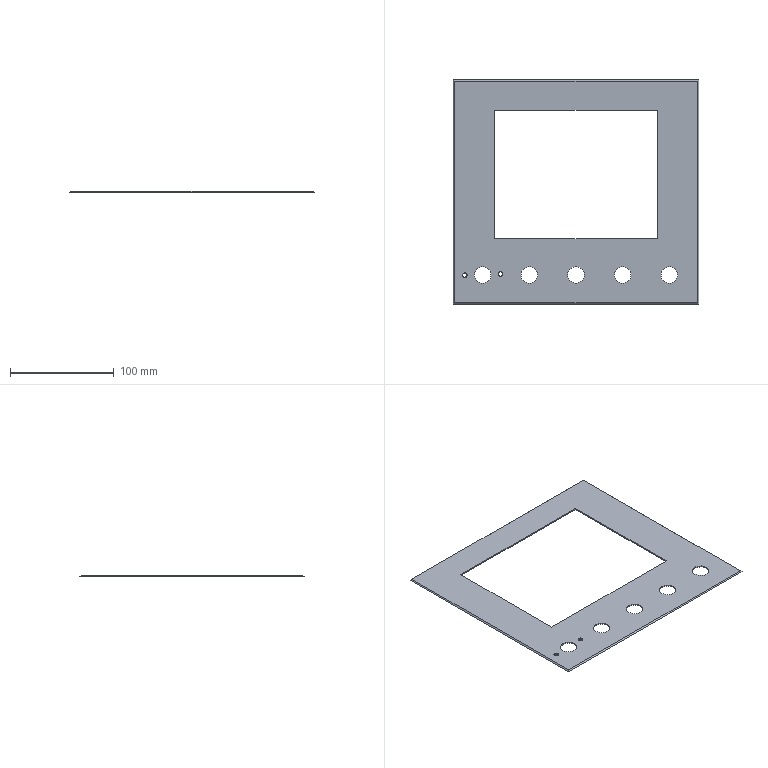Part | NX | 1 solid | 28 faces | box 236.4 x 216.4 x 1.2 mm | volume 36214 mm3 | cylinder 14 | plane 10 | cone 4 | commonest cylinder face diameters 16 x10 4 x4
STEP:
#1=CARTESIAN_POINT('',(-117.,-107.,75.));
#2=VERTEX_POINT('',#1);
#3=CARTESIAN_POINT('',(-117.,107.,75.));
#4=VERTEX_POINT('',#3);
#5=CARTESIAN_POINT('',(-117.,0.,75.));
#6=DIRECTION('',(0.,1.,0.));
#7=VECTOR('',#6,1000.);
#8=LINE('',#5,#7);
#9=EDGE_CURVE('',#2,#4,#8,.T.);
#10=ORIENTED_EDGE('',*,*,#9,.F.);
#11=CARTESIAN_POINT('',(117.,-107.,75.));
#12=VERTEX_POINT('',#11);
#13=CARTESIAN_POINT('',(0.,-107.,75.));
#14=DIRECTION('',(-1.,0.,0.));
#15=VECTOR('',#14,1000.);
#16=LINE('',#13,#15);
#17=EDGE_CURVE('',#12,#2,#16,.T.);
#18=ORIENTED_EDGE('',*,*,#17,.F.);
#19=CARTESIAN_POINT('',(117.,107.,75.));
#20=VERTEX_POINT('',#19);
#21=CARTESIAN_POINT('',(117.,0.,75.));
#22=DIRECTION('',(0.,-1.,0.));
#23=VECTOR('',#22,1000.);
#24=LINE('',#21,#23);
#25=EDGE_CURVE('',#20,#12,#24,.T.);
#26=ORIENTED_EDGE('',*,*,#25,.F.);
#27=CARTESIAN_POINT('',(0.,107.,75.));
#28=DIRECTION('',(-1.,0.,0.));
#29=VECTOR('',#28,1000.);
#30=LINE('',#27,#29);
#31=EDGE_CURVE('',#20,#4,#30,.T.);
#32=ORIENTED_EDGE('',*,*,#31,.T.);
#33=EDGE_LOOP('',(#10,#18,#26,#32));
#34=FACE_BOUND('',#33,.T.);
#35=CARTESIAN_POINT('',(-74.971,-79.122,75.));
#36=VERTEX_POINT('',#35);
#37=CARTESIAN_POINT('',(-70.571,-79.122,75.));
#38=VERTEX_POINT('',#37);
#39=CARTESIAN_POINT('',(-72.771,-79.122,75.));
#40=DIRECTION('',(0.,0.,1.));
#41=DIRECTION('',(1.,0.,0.));
#42=AXIS2_PLACEMENT_3D('',#39,#40,#41);
#43=CIRCLE('',#42,2.2);
#44=EDGE_CURVE('',#36,#38,#43,.T.);
#45=ORIENTED_EDGE('',*,*,#44,.F.);
#46=CARTESIAN_POINT('',(-72.771,-79.122,75.));
#47=DIRECTION('',(0.,0.,1.));
#48=DIRECTION('',(1.,0.,0.));
#49=AXIS2_PLACEMENT_3D('',#46,#47,#48);
#50=CIRCLE('',#49,2.2);
#51=EDGE_CURVE('',#38,#36,#50,.T.);
#52=ORIENTED_EDGE('',*,*,#51,.F.);
#53=EDGE_LOOP('',(#45,#52));
#54=FACE_BOUND('',#53,.T.);
#55=CARTESIAN_POINT('',(-98.,-80.,75.));
#56=VERTEX_POINT('',#55);
#57=CARTESIAN_POINT('',(-82.,-80.,75.));
#58=VERTEX_POINT('',#57);
#59=CARTESIAN_POINT('',(-90.,-80.,75.));
#60=DIRECTION('',(0.,0.,1.));
#61=DIRECTION('',(-1.,0.,0.));
#62=AXIS2_PLACEMENT_3D('',#59,#60,#61);
#63=CIRCLE('',#62,8.);
#64=EDGE_CURVE('',#56,#58,#63,.T.);
#65=ORIENTED_EDGE('',*,*,#64,.F.);
#66=CARTESIAN_POINT('',(-90.,-80.,75.));
#67=DIRECTION('',(0.,0.,1.));
#68=DIRECTION('',(-1.,0.,0.));
#69=AXIS2_PLACEMENT_3D('',#66,#67,#68);
#70=CIRCLE('',#69,8.);
#71=EDGE_CURVE('',#58,#56,#70,.T.);
#72=ORIENTED_EDGE('',*,*,#71,.F.);
#73=EDGE_LOOP('',(#65,#72));
#74=FACE_BOUND('',#73,.T.);
#75=CARTESIAN_POINT('',(-53.,-80.,75.));
#76=VERTEX_POINT('',#75);
#77=CARTESIAN_POINT('',(-37.,-80.,75.));
#78=VERTEX_POINT('',#77);
#79=CARTESIAN_POINT('',(-45.,-80.,75.));
#80=DIRECTION('',(0.,0.,1.));
#81=DIRECTION('',(-1.,0.,0.));
#82=AXIS2_PLACEMENT_3D('',#79,#80,#81);
#83=CIRCLE('',#82,8.);
#84=EDGE_CURVE('',#76,#78,#83,.T.);
#85=ORIENTED_EDGE('',*,*,#84,.F.);
#86=CARTESIAN_POINT('',(-45.,-80.,75.));
#87=DIRECTION('',(0.,0.,1.));
#88=DIRECTION('',(-1.,0.,0.));
#89=AXIS2_PLACEMENT_3D('',#86,#87,#88);
#90=CIRCLE('',#89,8.);
#91=EDGE_CURVE('',#78,#76,#90,.T.);
#92=ORIENTED_EDGE('',*,*,#91,.F.);
#93=EDGE_LOOP('',(#85,#92));
#94=FACE_BOUND('',#93,.T.);
#95=CARTESIAN_POINT('',(8.,-80.,75.));
#96=VERTEX_POINT('',#95);
#97=CARTESIAN_POINT('',(-8.,-80.,75.));
#98=VERTEX_POINT('',#97);
#99=CARTESIAN_POINT('',(0.,-80.,75.));
#100=DIRECTION('',(0.,0.,1.));
#101=DIRECTION('',(-1.,0.,0.));
#102=AXIS2_PLACEMENT_3D('',#99,#100,#101);
#103=CIRCLE('',#102,8.);
#104=EDGE_CURVE('',#96,#98,#103,.T.);
#105=ORIENTED_EDGE('',*,*,#104,.F.);
#106=CARTESIAN_POINT('',(0.,-80.,75.));
#107=DIRECTION('',(0.,0.,1.));
#108=DIRECTION('',(-1.,0.,0.));
#109=AXIS2_PLACEMENT_3D('',#106,#107,#108);
#110=CIRCLE('',#109,8.);
#111=EDGE_CURVE('',#98,#96,#110,.T.);
#112=ORIENTED_EDGE('',*,*,#111,.F.);
#113=EDGE_LOOP('',(#105,#112));
#114=FACE_BOUND('',#113,.T.);
#115=CARTESIAN_POINT('',(37.,-80.,75.));
#116=VERTEX_POINT('',#115);
#117=CARTESIAN_POINT('',(53.,-80.,75.));
#118=VERTEX_POINT('',#117);
#119=CARTESIAN_POINT('',(45.,-80.,75.));
#120=DIRECTION('',(0.,0.,1.));
#121=DIRECTION('',(-1.,0.,0.));
#122=AXIS2_PLACEMENT_3D('',#119,#120,#121);
#123=CIRCLE('',#122,8.);
#124=EDGE_CURVE('',#116,#118,#123,.T.);
#125=ORIENTED_EDGE('',*,*,#124,.F.);
#126=CARTESIAN_POINT('',(45.,-80.,75.));
#127=DIRECTION('',(0.,0.,1.));
#128=DIRECTION('',(-1.,0.,0.));
#129=AXIS2_PLACEMENT_3D('',#126,#127,#128);
#130=CIRCLE('',#129,8.);
#131=EDGE_CURVE('',#118,#116,#130,.T.);
#132=ORIENTED_EDGE('',*,*,#131,.F.);
#133=EDGE_LOOP('',(#125,#132));
#134=FACE_BOUND('',#133,.T.);
#135=CARTESIAN_POINT('',(98.,-80.,75.));
#136=VERTEX_POINT('',#135);
#137=CARTESIAN_POINT('',(82.,-80.,75.));
#138=VERTEX_POINT('',#137);
#139=CARTESIAN_POINT('',(90.,-80.,75.));
#140=DIRECTION('',(0.,0.,1.));
#141=DIRECTION('',(-1.,0.,0.));
#142=AXIS2_PLACEMENT_3D('',#139,#140,#141);
#143=CIRCLE('',#142,8.);
#144=EDGE_CURVE('',#136,#138,#143,.T.);
#145=ORIENTED_EDGE('',*,*,#144,.F.);
#146=CARTESIAN_POINT('',(90.,-80.,75.));
#147=DIRECTION('',(0.,0.,1.));
#148=DIRECTION('',(-1.,0.,0.));
#149=AXIS2_PLACEMENT_3D('',#146,#147,#148);
#150=CIRCLE('',#149,8.);
#151=EDGE_CURVE('',#138,#136,#150,.T.);
#152=ORIENTED_EDGE('',*,*,#151,.F.);
#153=EDGE_LOOP('',(#145,#152));
#154=FACE_BOUND('',#153,.T.);
#155=CARTESIAN_POINT('',(-109.448,-80.274,75.));
#156=VERTEX_POINT('',#155);
#157=CARTESIAN_POINT('',(-105.048,-80.274,75.));
#158=VERTEX_POINT('',#157);
#159=CARTESIAN_POINT('',(-107.248,-80.274,75.));
#160=DIRECTION('',(0.,0.,1.));
#161=DIRECTION('',(1.,0.,0.));
#162=AXIS2_PLACEMENT_3D('',#159,#160,#161);
#163=CIRCLE('',#162,2.2);
#164=EDGE_CURVE('',#156,#158,#163,.T.);
#165=ORIENTED_EDGE('',*,*,#164,.F.);
#166=CARTESIAN_POINT('',(-107.248,-80.274,75.));
#167=DIRECTION('',(0.,0.,1.));
#168=DIRECTION('',(1.,0.,0.));
#169=AXIS2_PLACEMENT_3D('',#166,#167,#168);
#170=CIRCLE('',#169,2.2);
#171=EDGE_CURVE('',#158,#156,#170,.T.);
#172=ORIENTED_EDGE('',*,*,#171,.F.);
#173=EDGE_LOOP('',(#165,#172));
#174=FACE_BOUND('',#173,.T.);
#175=CARTESIAN_POINT('',(-78.25,-45.,75.));
#176=VERTEX_POINT('',#175);
#177=CARTESIAN_POINT('',(-78.25,79.,75.));
#178=VERTEX_POINT('',#177);
#179=CARTESIAN_POINT('',(-78.25,-45.,75.));
#180=DIRECTION('',(0.,1.,0.));
#181=VECTOR('',#180,1000.);
#182=LINE('',#179,#181);
#183=EDGE_CURVE('',#176,#178,#182,.T.);
#184=ORIENTED_EDGE('',*,*,#183,.T.);
#185=CARTESIAN_POINT('',(78.25,79.,75.));
#186=VERTEX_POINT('',#185);
#187=CARTESIAN_POINT('',(-78.25,79.,75.));
#188=DIRECTION('',(1.,0.,0.));
#189=VECTOR('',#188,1000.);
#190=LINE('',#187,#189);
#191=EDGE_CURVE('',#178,#186,#190,.T.);
#192=ORIENTED_EDGE('',*,*,#191,.T.);
#193=CARTESIAN_POINT('',(78.25,-45.,75.));
#194=VERTEX_POINT('',#193);
#195=CARTESIAN_POINT('',(78.25,79.,75.));
#196=DIRECTION('',(0.,-1.,0.));
#197=VECTOR('',#196,1000.);
#198=LINE('',#195,#197);
#199=EDGE_CURVE('',#186,#194,#198,.T.);
#200=ORIENTED_EDGE('',*,*,#199,.T.);
#201=CARTESIAN_POINT('',(78.25,-45.,75.));
#202=DIRECTION('',(-1.,0.,0.));
#203=VECTOR('',#202,1000.);
#204=LINE('',#201,#203);
#205=EDGE_CURVE('',#194,#176,#204,.T.);
#206=ORIENTED_EDGE('',*,*,#205,.T.);
#207=EDGE_LOOP('',(#184,#192,#200,#206));
#208=FACE_BOUND('',#207,.T.);
#209=CARTESIAN_POINT('',(0.,0.,75.));
#210=DIRECTION('',(0.,0.,1.));
#211=DIRECTION('',(1.,0.,0.));
#212=AXIS2_PLACEMENT_3D('',#209,#210,#211);
#213=PLANE('',#212);
#214=ADVANCED_FACE('',(#34,#54,#74,#94,#114,#134,#154,#174,#208),#213,.T.);
#215=CARTESIAN_POINT('',(-74.771,-79.122,74.8));
#216=VERTEX_POINT('',#215);
#217=CARTESIAN_POINT('',(-70.771,-79.122,74.8));
#218=VERTEX_POINT('',#217);
#219=CARTESIAN_POINT('',(-72.771,-79.122,74.8));
#220=DIRECTION('',(0.,0.,1.));
#221=DIRECTION('',(1.,0.,0.));
#222=AXIS2_PLACEMENT_3D('',#219,#220,#221);
#223=CIRCLE('',#222,2.);
#224=EDGE_CURVE('',#216,#218,#223,.T.);
#225=ORIENTED_EDGE('',*,*,#224,.F.);
#226=CARTESIAN_POINT('',(-74.771,-79.122,74.8));
#227=DIRECTION('',(-0.7071,0.,0.7071));
#228=VECTOR('',#227,1000.);
#229=LINE('',#226,#228);
#230=EDGE_CURVE('',#216,#36,#229,.T.);
#231=ORIENTED_EDGE('',*,*,#230,.T.);
#232=ORIENTED_EDGE('',*,*,#44,.T.);
#233=CARTESIAN_POINT('',(-70.771,-79.122,74.8));
#234=DIRECTION('',(0.7071,0.,0.7071));
#235=VECTOR('',#234,1000.);
#236=LINE('',#233,#235);
#237=EDGE_CURVE('',#218,#38,#236,.T.);
#238=ORIENTED_EDGE('',*,*,#237,.F.);
#239=EDGE_LOOP('',(#225,#231,#232,#238));
#240=FACE_BOUND('',#239,.T.);
#241=CARTESIAN_POINT('',(-72.771,-79.122,74.8));
#242=DIRECTION('',(0.,0.,1.));
#243=DIRECTION('',(1.,0.,0.));
#244=AXIS2_PLACEMENT_3D('',#241,#242,#243);
#245=CONICAL_SURFACE('',#244,2.,0.7854);
#246=ADVANCED_FACE('',(#240),#245,.F.);
#247=ORIENTED_EDGE('',*,*,#224,.T.);
#248=CARTESIAN_POINT('',(-70.771,-79.122,73.8));
#249=VERTEX_POINT('',#248);
#250=CARTESIAN_POINT('',(-70.771,-79.122,75.));
#251=DIRECTION('',(0.,0.,1.));
#252=VECTOR('',#251,1000.);
#253=LINE('',#250,#252);
#254=EDGE_CURVE('',#249,#218,#253,.T.);
#255=ORIENTED_EDGE('',*,*,#254,.F.);
#256=CARTESIAN_POINT('',(-74.771,-79.122,73.8));
#257=VERTEX_POINT('',#256);
#258=CARTESIAN_POINT('',(-72.771,-79.122,73.8));
#259=DIRECTION('',(0.,0.,1.));
#260=DIRECTION('',(1.,0.,0.));
#261=AXIS2_PLACEMENT_3D('',#258,#259,#260);
#262=CIRCLE('',#261,2.);
#263=EDGE_CURVE('',#257,#249,#262,.T.);
#264=ORIENTED_EDGE('',*,*,#263,.F.);
#265=CARTESIAN_POINT('',(-74.771,-79.122,75.));
#266=DIRECTION('',(0.,0.,1.));
#267=VECTOR('',#266,1000.);
#268=LINE('',#265,#267);
#269=EDGE_CURVE('',#257,#216,#268,.T.);
#270=ORIENTED_EDGE('',*,*,#269,.T.);
#271=EDGE_LOOP('',(#247,#255,#264,#270));
#272=FACE_BOUND('',#271,.T.);
#273=CARTESIAN_POINT('',(-72.771,-79.122,75.));
#274=DIRECTION('',(0.,0.,1.));
#275=DIRECTION('',(1.,0.,0.));
#276=AXIS2_PLACEMENT_3D('',#273,#274,#275);
#277=CYLINDRICAL_SURFACE('',#276,2.);
#278=ADVANCED_FACE('',(#272),#277,.F.);
#279=CARTESIAN_POINT('',(-118.2,108.2,73.8));
#280=VERTEX_POINT('',#279);
#281=CARTESIAN_POINT('',(118.2,108.2,73.8));
#282=VERTEX_POINT('',#281);
#283=CARTESIAN_POINT('',(0.,108.2,73.8));
#284=DIRECTION('',(1.,0.,0.));
#285=VECTOR('',#284,1000.);
#286=LINE('',#283,#285);
#287=EDGE_CURVE('',#280,#282,#286,.T.);
#288=ORIENTED_EDGE('',*,*,#287,.T.);
#289=CARTESIAN_POINT('',(118.2,-108.2,73.8));
#290=VERTEX_POINT('',#289);
#291=CARTESIAN_POINT('',(118.2,0.,73.8));
#292=DIRECTION('',(0.,-1.,0.));
#293=VECTOR('',#292,1000.);
#294=LINE('',#291,#293);
#295=EDGE_CURVE('',#282,#290,#294,.T.);
#296=ORIENTED_EDGE('',*,*,#295,.T.);
#297=CARTESIAN_POINT('',(-118.2,-108.2,73.8));
#298=VERTEX_POINT('',#297);
#299=CARTESIAN_POINT('',(0.,-108.2,73.8));
#300=DIRECTION('',(1.,0.,0.));
#301=VECTOR('',#300,1000.);
#302=LINE('',#299,#301);
#303=EDGE_CURVE('',#298,#290,#302,.T.);
#304=ORIENTED_EDGE('',*,*,#303,.F.);
#305=CARTESIAN_POINT('',(-118.2,0.,73.8));
#306=DIRECTION('',(0.,1.,0.));
#307=VECTOR('',#306,1000.);
#308=LINE('',#305,#307);
#309=EDGE_CURVE('',#298,#280,#308,.T.);
#310=ORIENTED_EDGE('',*,*,#309,.T.);
#311=EDGE_LOOP('',(#288,#296,#304,#310));
#312=FACE_BOUND('',#311,.T.);
#313=CARTESIAN_POINT('',(98.,-80.,73.8));
#314=VERTEX_POINT('',#313);
#315=CARTESIAN_POINT('',(82.,-80.,73.8));
#316=VERTEX_POINT('',#315);
#317=CARTESIAN_POINT('',(90.,-80.,73.8));
#318=DIRECTION('',(0.,0.,-1.));
#319=DIRECTION('',(1.,0.,0.));
#320=AXIS2_PLACEMENT_3D('',#317,#318,#319);
#321=CIRCLE('',#320,8.);
#322=EDGE_CURVE('',#314,#316,#321,.T.);
#323=ORIENTED_EDGE('',*,*,#322,.F.);
#324=CARTESIAN_POINT('',(90.,-80.,73.8));
#325=DIRECTION('',(0.,0.,-1.));
#326=DIRECTION('',(1.,0.,0.));
#327=AXIS2_PLACEMENT_3D('',#324,#325,#326);
#328=CIRCLE('',#327,8.);
#329=EDGE_CURVE('',#316,#314,#328,.T.);
#330=ORIENTED_EDGE('',*,*,#329,.F.);
#331=EDGE_LOOP('',(#323,#330));
#332=FACE_BOUND('',#331,.T.);
#333=CARTESIAN_POINT('',(-109.248,-80.274,73.8));
#334=VERTEX_POINT('',#333);
#335=CARTESIAN_POINT('',(-105.248,-80.274,73.8));
#336=VERTEX_POINT('',#335);
#337=CARTESIAN_POINT('',(-107.248,-80.274,73.8));
#338=DIRECTION('',(0.,0.,1.));
#339=DIRECTION('',(1.,0.,0.));
#340=AXIS2_PLACEMENT_3D('',#337,#338,#339);
#341=CIRCLE('',#340,2.);
#342=EDGE_CURVE('',#334,#336,#341,.T.);
#343=ORIENTED_EDGE('',*,*,#342,.T.);
#344=CARTESIAN_POINT('',(-107.248,-80.274,73.8));
#345=DIRECTION('',(0.,0.,1.));
#346=DIRECTION('',(1.,0.,0.));
#347=AXIS2_PLACEMENT_3D('',#344,#345,#346);
#348=CIRCLE('',#347,2.);
#349=EDGE_CURVE('',#336,#334,#348,.T.);
#350=ORIENTED_EDGE('',*,*,#349,.T.);
#351=EDGE_LOOP('',(#343,#350));
#352=FACE_BOUND('',#351,.T.);
#353=ORIENTED_EDGE('',*,*,#263,.T.);
#354=CARTESIAN_POINT('',(-72.771,-79.122,73.8));
#355=DIRECTION('',(0.,0.,1.));
#356=DIRECTION('',(1.,0.,0.));
#357=AXIS2_PLACEMENT_3D('',#354,#355,#356);
#358=CIRCLE('',#357,2.);
#359=EDGE_CURVE('',#249,#257,#358,.T.);
#360=ORIENTED_EDGE('',*,*,#359,.T.);
#361=EDGE_LOOP('',(#353,#360));
#362=FACE_BOUND('',#361,.T.);
#363=CARTESIAN_POINT('',(-78.25,-45.,73.8));
#364=VERTEX_POINT('',#363);
#365=CARTESIAN_POINT('',(-78.25,79.,73.8));
#366=VERTEX_POINT('',#365);
#367=CARTESIAN_POINT('',(-78.25,-45.,73.8));
#368=DIRECTION('',(0.,1.,0.));
#369=VECTOR('',#368,1000.);
#370=LINE('',#367,#369);
#371=EDGE_CURVE('',#364,#366,#370,.T.);
#372=ORIENTED_EDGE('',*,*,#371,.F.);
#373=CARTESIAN_POINT('',(78.25,-45.,73.8));
#374=VERTEX_POINT('',#373);
#375=CARTESIAN_POINT('',(78.25,-45.,73.8));
#376=DIRECTION('',(-1.,0.,0.));
#377=VECTOR('',#376,1000.);
#378=LINE('',#375,#377);
#379=EDGE_CURVE('',#374,#364,#378,.T.);
#380=ORIENTED_EDGE('',*,*,#379,.F.);
#381=CARTESIAN_POINT('',(78.25,79.,73.8));
#382=VERTEX_POINT('',#381);
#383=CARTESIAN_POINT('',(78.25,79.,73.8));
#384=DIRECTION('',(0.,-1.,0.));
#385=VECTOR('',#384,1000.);
#386=LINE('',#383,#385);
#387=EDGE_CURVE('',#382,#374,#386,.T.);
#388=ORIENTED_EDGE('',*,*,#387,.F.);
#389=CARTESIAN_POINT('',(-78.25,79.,73.8));
#390=DIRECTION('',(1.,0.,0.));
#391=VECTOR('',#390,1000.);
#392=LINE('',#389,#391);
#393=EDGE_CURVE('',#366,#382,#392,.T.);
#394=ORIENTED_EDGE('',*,*,#393,.F.);
#395=EDGE_LOOP('',(#372,#380,#388,#394));
#396=FACE_BOUND('',#395,.T.);
#397=CARTESIAN_POINT('',(-98.,-80.,73.8));
#398=VERTEX_POINT('',#397);
#399=CARTESIAN_POINT('',(-82.,-80.,73.8));
#400=VERTEX_POINT('',#399);
#401=CARTESIAN_POINT('',(-90.,-80.,73.8));
#402=DIRECTION('',(0.,0.,-1.));
#403=DIRECTION('',(1.,0.,0.));
#404=AXIS2_PLACEMENT_3D('',#401,#402,#403);
#405=CIRCLE('',#404,8.);
#406=EDGE_CURVE('',#398,#400,#405,.T.);
#407=ORIENTED_EDGE('',*,*,#406,.F.);
#408=CARTESIAN_POINT('',(-90.,-80.,73.8));
#409=DIRECTION('',(0.,0.,-1.));
#410=DIRECTION('',(1.,0.,0.));
#411=AXIS2_PLACEMENT_3D('',#408,#409,#410);
#412=CIRCLE('',#411,8.);
#413=EDGE_CURVE('',#400,#398,#412,.T.);
#414=ORIENTED_EDGE('',*,*,#413,.F.);
#415=EDGE_LOOP('',(#407,#414));
#416=FACE_BOUND('',#415,.T.);
#417=CARTESIAN_POINT('',(-37.,-80.,73.8));
#418=VERTEX_POINT('',#417);
#419=CARTESIAN_POINT('',(-53.,-80.,73.8));
#420=VERTEX_POINT('',#419);
#421=CARTESIAN_POINT('',(-45.,-80.,73.8));
#422=DIRECTION('',(0.,0.,-1.));
#423=DIRECTION('',(1.,0.,0.));
#424=AXIS2_PLACEMENT_3D('',#421,#422,#423);
#425=CIRCLE('',#424,8.);
#426=EDGE_CURVE('',#418,#420,#425,.T.);
#427=ORIENTED_EDGE('',*,*,#426,.F.);
#428=CARTESIAN_POINT('',(-45.,-80.,73.8));
#429=DIRECTION('',(0.,0.,-1.));
#430=DIRECTION('',(1.,0.,0.));
#431=AXIS2_PLACEMENT_3D('',#428,#429,#430);
#432=CIRCLE('',#431,8.);
#433=EDGE_CURVE('',#420,#418,#432,.T.);
#434=ORIENTED_EDGE('',*,*,#433,.F.);
#435=EDGE_LOOP('',(#427,#434));
#436=FACE_BOUND('',#435,.T.);
#437=CARTESIAN_POINT('',(8.,-80.,73.8));
#438=VERTEX_POINT('',#437);
#439=CARTESIAN_POINT('',(-8.,-80.,73.8));
#440=VERTEX_POINT('',#439);
#441=CARTESIAN_POINT('',(0.,-80.,73.8));
#442=DIRECTION('',(0.,0.,-1.));
#443=DIRECTION('',(1.,0.,0.));
#444=AXIS2_PLACEMENT_3D('',#441,#442,#443);
#445=CIRCLE('',#444,8.);
#446=EDGE_CURVE('',#438,#440,#445,.T.);
#447=ORIENTED_EDGE('',*,*,#446,.F.);
#448=CARTESIAN_POINT('',(0.,-80.,73.8));
#449=DIRECTION('',(0.,0.,-1.));
#450=DIRECTION('',(1.,0.,0.));
#451=AXIS2_PLACEMENT_3D('',#448,#449,#450);
#452=CIRCLE('',#451,8.);
#453=EDGE_CURVE('',#440,#438,#452,.T.);
#454=ORIENTED_EDGE('',*,*,#453,.F.);
#455=EDGE_LOOP('',(#447,#454));
#456=FACE_BOUND('',#455,.T.);
#457=CARTESIAN_POINT('',(37.,-80.,73.8));
#458=VERTEX_POINT('',#457);
#459=CARTESIAN_POINT('',(53.,-80.,73.8));
#460=VERTEX_POINT('',#459);
#461=CARTESIAN_POINT('',(45.,-80.,73.8));
#462=DIRECTION('',(0.,0.,-1.));
#463=DIRECTION('',(1.,0.,0.));
#464=AXIS2_PLACEMENT_3D('',#461,#462,#463);
#465=CIRCLE('',#464,8.);
#466=EDGE_CURVE('',#458,#460,#465,.T.);
#467=ORIENTED_EDGE('',*,*,#466,.F.);
#468=CARTESIAN_POINT('',(45.,-80.,73.8));
#469=DIRECTION('',(0.,0.,-1.));
#470=DIRECTION('',(1.,0.,0.));
#471=AXIS2_PLACEMENT_3D('',#468,#469,#470);
#472=CIRCLE('',#471,8.);
#473=EDGE_CURVE('',#460,#458,#472,.T.);
#474=ORIENTED_EDGE('',*,*,#473,.F.);
#475=EDGE_LOOP('',(#467,#474));
#476=FACE_BOUND('',#475,.T.);
#477=CARTESIAN_POINT('',(0.,0.,73.8));
#478=DIRECTION('',(0.,0.,1.));
#479=DIRECTION('',(1.,0.,0.));
#480=AXIS2_PLACEMENT_3D('',#477,#478,#479);
#481=PLANE('',#480);
#482=ADVANCED_FACE('',(#312,#332,#352,#362,#396,#416,#436,#456,#476),#481,.F.);
#483=ORIENTED_EDGE('',*,*,#303,.T.);
#484=CARTESIAN_POINT('',(192.,-182.,0.));
#485=DIRECTION('',(0.5774,-0.5774,-0.5774));
#486=VECTOR('',#485,1000.);
#487=LINE('',#484,#486);
#488=EDGE_CURVE('',#12,#290,#487,.T.);
#489=ORIENTED_EDGE('',*,*,#488,.F.);
#490=ORIENTED_EDGE('',*,*,#17,.T.);
#491=CARTESIAN_POINT('',(-192.,-182.,0.));
#492=DIRECTION('',(-0.5774,-0.5774,-0.5774));
#493=VECTOR('',#492,1000.);
#494=LINE('',#491,#493);
#495=EDGE_CURVE('',#2,#298,#494,.T.);
#496=ORIENTED_EDGE('',*,*,#495,.T.);
#497=EDGE_LOOP('',(#483,#489,#490,#496));
#498=FACE_BOUND('',#497,.T.);
#499=CARTESIAN_POINT('',(0.,-108.5,73.5));
#500=DIRECTION('',(0.,-0.7071,0.7071));
#501=DIRECTION('',(-1.,0.,0.));
#502=AXIS2_PLACEMENT_3D('',#499,#500,#501);
#503=PLANE('',#502);
#504=ADVANCED_FACE('',(#498),#503,.T.);
#505=ORIENTED_EDGE('',*,*,#9,.T.);
#506=CARTESIAN_POINT('',(-192.,182.,0.));
#507=DIRECTION('',(-0.5774,0.5774,-0.5774));
#508=VECTOR('',#507,1000.);
#509=LINE('',#506,#508);
#510=EDGE_CURVE('',#4,#280,#509,.T.);
#511=ORIENTED_EDGE('',*,*,#510,.T.);
#512=ORIENTED_EDGE('',*,*,#309,.F.);
#513=ORIENTED_EDGE('',*,*,#495,.F.);
#514=EDGE_LOOP('',(#505,#511,#512,#513));
#515=FACE_BOUND('',#514,.T.);
#516=CARTESIAN_POINT('',(-118.5,0.,73.5));
#517=DIRECTION('',(0.7071,0.,-0.7071));
#518=DIRECTION('',(0.,-1.,0.));
#519=AXIS2_PLACEMENT_3D('',#516,#517,#518);
#520=PLANE('',#519);
#521=ADVANCED_FACE('',(#515),#520,.F.);
#522=ORIENTED_EDGE('',*,*,#25,.T.);
#523=ORIENTED_EDGE('',*,*,#488,.T.);
#524=ORIENTED_EDGE('',*,*,#295,.F.);
#525=CARTESIAN_POINT('',(192.,182.,0.));
#526=DIRECTION('',(-0.5774,-0.5774,0.5774));
#527=VECTOR('',#526,1000.);
#528=LINE('',#525,#527);
#529=EDGE_CURVE('',#282,#20,#528,.T.);
#530=ORIENTED_EDGE('',*,*,#529,.T.);
#531=EDGE_LOOP('',(#522,#523,#524,#530));
#532=FACE_BOUND('',#531,.T.);
#533=CARTESIAN_POINT('',(118.5,0.,73.5));
#534=DIRECTION('',(-0.7071,0.,-0.7071));
#535=DIRECTION('',(-0.7071,0.,0.7071));
#536=AXIS2_PLACEMENT_3D('',#533,#534,#535);
#537=PLANE('',#536);
#538=ADVANCED_FACE('',(#532),#537,.F.);
#539=ORIENTED_EDGE('',*,*,#287,.F.);
#540=ORIENTED_EDGE('',*,*,#510,.F.);
#541=ORIENTED_EDGE('',*,*,#31,.F.);
#542=ORIENTED_EDGE('',*,*,#529,.F.);
#543=EDGE_LOOP('',(#539,#540,#541,#542));
#544=FACE_BOUND('',#543,.T.);
#545=CARTESIAN_POINT('',(0.,108.5,73.5));
#546=DIRECTION('',(0.,-0.7071,-0.7071));
#547=DIRECTION('',(0.,-0.7071,0.7071));
#548=AXIS2_PLACEMENT_3D('',#545,#546,#547);
#549=PLANE('',#548);
#550=ADVANCED_FACE('',(#544),#549,.F.);
#551=ORIENTED_EDGE('',*,*,#322,.T.);
#552=CARTESIAN_POINT('',(82.,-80.,75.));
#553=DIRECTION('',(0.,0.,-1.));
#554=VECTOR('',#553,1000.);
#555=LINE('',#552,#554);
#556=EDGE_CURVE('',#316,#138,#555,.F.);
#557=ORIENTED_EDGE('',*,*,#556,.T.);
#558=ORIENTED_EDGE('',*,*,#151,.T.);
#559=CARTESIAN_POINT('',(98.,-80.,75.));
#560=DIRECTION('',(0.,0.,-1.));
#561=VECTOR('',#560,1000.);
#562=LINE('',#559,#561);
#563=EDGE_CURVE('',#314,#136,#562,.F.);
#564=ORIENTED_EDGE('',*,*,#563,.F.);
#565=EDGE_LOOP('',(#551,#557,#558,#564));
#566=FACE_BOUND('',#565,.T.);
#567=CARTESIAN_POINT('',(90.,-80.,75.));
#568=DIRECTION('',(0.,0.,-1.));
#569=DIRECTION('',(-1.,0.,0.));
#570=AXIS2_PLACEMENT_3D('',#567,#568,#569);
#571=CYLINDRICAL_SURFACE('',#570,8.);
#572=ADVANCED_FACE('',(#566),#571,.F.);
#573=CARTESIAN_POINT('',(-109.248,-80.274,74.8));
#574=VERTEX_POINT('',#573);
#575=CARTESIAN_POINT('',(-105.248,-80.274,74.8));
#576=VERTEX_POINT('',#575);
#577=CARTESIAN_POINT('',(-107.248,-80.274,74.8));
#578=DIRECTION('',(0.,0.,1.));
#579=DIRECTION('',(1.,0.,0.));
#580=AXIS2_PLACEMENT_3D('',#577,#578,#579);
#581=CIRCLE('',#580,2.);
#582=EDGE_CURVE('',#574,#576,#581,.T.);
#583=ORIENTED_EDGE('',*,*,#582,.T.);
#584=CARTESIAN_POINT('',(-105.248,-80.274,75.));
#585=DIRECTION('',(0.,0.,1.));
#586=VECTOR('',#585,1000.);
#587=LINE('',#584,#586);
#588=EDGE_CURVE('',#336,#576,#587,.T.);
#589=ORIENTED_EDGE('',*,*,#588,.F.);
#590=ORIENTED_EDGE('',*,*,#342,.F.);
#591=CARTESIAN_POINT('',(-109.248,-80.274,75.));
#592=DIRECTION('',(0.,0.,1.));
#593=VECTOR('',#592,1000.);
#594=LINE('',#591,#593);
#595=EDGE_CURVE('',#334,#574,#594,.T.);
#596=ORIENTED_EDGE('',*,*,#595,.T.);
#597=EDGE_LOOP('',(#583,#589,#590,#596));
#598=FACE_BOUND('',#597,.T.);
#599=CARTESIAN_POINT('',(-107.248,-80.274,75.));
#600=DIRECTION('',(0.,0.,1.));
#601=DIRECTION('',(1.,0.,0.));
#602=AXIS2_PLACEMENT_3D('',#599,#600,#601);
#603=CYLINDRICAL_SURFACE('',#602,2.);
#604=ADVANCED_FACE('',(#598),#603,.F.);
#605=ORIENTED_EDGE('',*,*,#582,.F.);
#606=CARTESIAN_POINT('',(-109.248,-80.274,74.8));
#607=DIRECTION('',(-0.7071,0.,0.7071));
#608=VECTOR('',#607,1000.);
#609=LINE('',#606,#608);
#610=EDGE_CURVE('',#574,#156,#609,.T.);
#611=ORIENTED_EDGE('',*,*,#610,.T.);
#612=ORIENTED_EDGE('',*,*,#164,.T.);
#613=CARTESIAN_POINT('',(-105.248,-80.274,74.8));
#614=DIRECTION('',(0.7071,0.,0.7071));
#615=VECTOR('',#614,1000.);
#616=LINE('',#613,#615);
#617=EDGE_CURVE('',#576,#158,#616,.T.);
#618=ORIENTED_EDGE('',*,*,#617,.F.);
#619=EDGE_LOOP('',(#605,#611,#612,#618));
#620=FACE_BOUND('',#619,.T.);
#621=CARTESIAN_POINT('',(-107.248,-80.274,74.8));
#622=DIRECTION('',(0.,0.,1.));
#623=DIRECTION('',(1.,0.,0.));
#624=AXIS2_PLACEMENT_3D('',#621,#622,#623);
#625=CONICAL_SURFACE('',#624,2.,0.7854);
#626=ADVANCED_FACE('',(#620),#625,.F.);
#627=ORIENTED_EDGE('',*,*,#371,.T.);
#628=CARTESIAN_POINT('',(-78.25,79.,73.8));
#629=DIRECTION('',(0.,0.,1.));
#630=VECTOR('',#629,1000.);
#631=LINE('',#628,#630);
#632=EDGE_CURVE('',#366,#178,#631,.T.);
#633=ORIENTED_EDGE('',*,*,#632,.T.);
#634=ORIENTED_EDGE('',*,*,#183,.F.);
#635=CARTESIAN_POINT('',(-78.25,-45.,73.8));
#636=DIRECTION('',(0.,0.,1.));
#637=VECTOR('',#636,1000.);
#638=LINE('',#635,#637);
#639=EDGE_CURVE('',#364,#176,#638,.T.);
#640=ORIENTED_EDGE('',*,*,#639,.F.);
#641=EDGE_LOOP('',(#627,#633,#634,#640));
#642=FACE_BOUND('',#641,.T.);
#643=CARTESIAN_POINT('',(-78.25,79.,75.));
#644=DIRECTION('',(-1.,0.,0.));
#645=DIRECTION('',(0.,0.,1.));
#646=AXIS2_PLACEMENT_3D('',#643,#644,#645);
#647=PLANE('',#646);
#648=ADVANCED_FACE('',(#642),#647,.F.);
#649=ORIENTED_EDGE('',*,*,#393,.T.);
#650=CARTESIAN_POINT('',(78.25,79.,73.8));
#651=DIRECTION('',(0.,0.,1.));
#652=VECTOR('',#651,1000.);
#653=LINE('',#650,#652);
#654=EDGE_CURVE('',#382,#186,#653,.T.);
#655=ORIENTED_EDGE('',*,*,#654,.T.);
#656=ORIENTED_EDGE('',*,*,#191,.F.);
#657=ORIENTED_EDGE('',*,*,#632,.F.);
#658=EDGE_LOOP('',(#649,#655,#656,#657));
#659=FACE_BOUND('',#658,.T.);
#660=CARTESIAN_POINT('',(78.25,79.,75.));
#661=DIRECTION('',(0.,1.,0.));
#662=DIRECTION('',(1.,0.,0.));
#663=AXIS2_PLACEMENT_3D('',#660,#661,#662);
#664=PLANE('',#663);
#665=ADVANCED_FACE('',(#659),#664,.F.);
#666=ORIENTED_EDGE('',*,*,#387,.T.);
#667=CARTESIAN_POINT('',(78.25,-45.,73.8));
#668=DIRECTION('',(0.,0.,1.));
#669=VECTOR('',#668,1000.);
#670=LINE('',#667,#669);
#671=EDGE_CURVE('',#374,#194,#670,.T.);
#672=ORIENTED_EDGE('',*,*,#671,.T.);
#673=ORIENTED_EDGE('',*,*,#199,.F.);
#674=ORIENTED_EDGE('',*,*,#654,.F.);
#675=EDGE_LOOP('',(#666,#672,#673,#674));
#676=FACE_BOUND('',#675,.T.);
#677=CARTESIAN_POINT('',(78.25,-45.,75.));
#678=DIRECTION('',(1.,0.,0.));
#679=DIRECTION('',(0.,1.,0.));
#680=AXIS2_PLACEMENT_3D('',#677,#678,#679);
#681=PLANE('',#680);
#682=ADVANCED_FACE('',(#676),#681,.F.);
#683=ORIENTED_EDGE('',*,*,#379,.T.);
#684=ORIENTED_EDGE('',*,*,#639,.T.);
#685=ORIENTED_EDGE('',*,*,#205,.F.);
#686=ORIENTED_EDGE('',*,*,#671,.F.);
#687=EDGE_LOOP('',(#683,#684,#685,#686));
#688=FACE_BOUND('',#687,.T.);
#689=CARTESIAN_POINT('',(-78.25,-45.,75.));
#690=DIRECTION('',(0.,-1.,0.));
#691=DIRECTION('',(0.,0.,-1.));
#692=AXIS2_PLACEMENT_3D('',#689,#690,#691);
#693=PLANE('',#692);
#694=ADVANCED_FACE('',(#688),#693,.F.);
#695=ORIENTED_EDGE('',*,*,#406,.T.);
#696=CARTESIAN_POINT('',(-82.,-80.,75.));
#697=DIRECTION('',(0.,0.,-1.));
#698=VECTOR('',#697,1000.);
#699=LINE('',#696,#698);
#700=EDGE_CURVE('',#58,#400,#699,.T.);
#701=ORIENTED_EDGE('',*,*,#700,.F.);
#702=ORIENTED_EDGE('',*,*,#71,.T.);
#703=CARTESIAN_POINT('',(-98.,-80.,75.));
#704=DIRECTION('',(0.,0.,-1.));
#705=VECTOR('',#704,1000.);
#706=LINE('',#703,#705);
#707=EDGE_CURVE('',#56,#398,#706,.T.);
#708=ORIENTED_EDGE('',*,*,#707,.T.);
#709=EDGE_LOOP('',(#695,#701,#702,#708));
#710=FACE_BOUND('',#709,.T.);
#711=CARTESIAN_POINT('',(-90.,-80.,75.));
#712=DIRECTION('',(0.,0.,-1.));
#713=DIRECTION('',(-1.,0.,0.));
#714=AXIS2_PLACEMENT_3D('',#711,#712,#713);
#715=CYLINDRICAL_SURFACE('',#714,8.);
#716=ADVANCED_FACE('',(#710),#715,.F.);
#717=ORIENTED_EDGE('',*,*,#426,.T.);
#718=CARTESIAN_POINT('',(-53.,-80.,75.));
#719=DIRECTION('',(0.,0.,-1.));
#720=VECTOR('',#719,1000.);
#721=LINE('',#718,#720);
#722=EDGE_CURVE('',#420,#76,#721,.F.);
#723=ORIENTED_EDGE('',*,*,#722,.T.);
#724=ORIENTED_EDGE('',*,*,#84,.T.);
#725=CARTESIAN_POINT('',(-37.,-80.,75.));
#726=DIRECTION('',(0.,0.,-1.));
#727=VECTOR('',#726,1000.);
#728=LINE('',#725,#727);
#729=EDGE_CURVE('',#418,#78,#728,.F.);
#730=ORIENTED_EDGE('',*,*,#729,.F.);
#731=EDGE_LOOP('',(#717,#723,#724,#730));
#732=FACE_BOUND('',#731,.T.);
#733=CARTESIAN_POINT('',(-45.,-80.,75.));
#734=DIRECTION('',(0.,0.,-1.));
#735=DIRECTION('',(-1.,0.,0.));
#736=AXIS2_PLACEMENT_3D('',#733,#734,#735);
#737=CYLINDRICAL_SURFACE('',#736,8.);
#738=ADVANCED_FACE('',(#732),#737,.F.);
#739=ORIENTED_EDGE('',*,*,#446,.T.);
#740=CARTESIAN_POINT('',(-8.,-80.,75.));
#741=DIRECTION('',(0.,0.,-1.));
#742=VECTOR('',#741,1000.);
#743=LINE('',#740,#742);
#744=EDGE_CURVE('',#440,#98,#743,.F.);
#745=ORIENTED_EDGE('',*,*,#744,.T.);
#746=ORIENTED_EDGE('',*,*,#111,.T.);
#747=CARTESIAN_POINT('',(8.,-80.,75.));
#748=DIRECTION('',(0.,0.,-1.));
#749=VECTOR('',#748,1000.);
#750=LINE('',#747,#749);
#751=EDGE_CURVE('',#438,#96,#750,.F.);
#752=ORIENTED_EDGE('',*,*,#751,.F.);
#753=EDGE_LOOP('',(#739,#745,#746,#752));
#754=FACE_BOUND('',#753,.T.);
#755=CARTESIAN_POINT('',(0.,-80.,75.));
#756=DIRECTION('',(0.,0.,-1.));
#757=DIRECTION('',(-1.,0.,0.));
#758=AXIS2_PLACEMENT_3D('',#755,#756,#757);
#759=CYLINDRICAL_SURFACE('',#758,8.);
#760=ADVANCED_FACE('',(#754),#759,.F.);
#761=ORIENTED_EDGE('',*,*,#466,.T.);
#762=CARTESIAN_POINT('',(53.,-80.,75.));
#763=DIRECTION('',(0.,0.,-1.));
#764=VECTOR('',#763,1000.);
#765=LINE('',#762,#764);
#766=EDGE_CURVE('',#118,#460,#765,.T.);
#767=ORIENTED_EDGE('',*,*,#766,.F.);
#768=ORIENTED_EDGE('',*,*,#131,.T.);
#769=CARTESIAN_POINT('',(37.,-80.,75.));
#770=DIRECTION('',(0.,0.,-1.));
#771=VECTOR('',#770,1000.);
#772=LINE('',#769,#771);
#773=EDGE_CURVE('',#116,#458,#772,.T.);
#774=ORIENTED_EDGE('',*,*,#773,.T.);
#775=EDGE_LOOP('',(#761,#767,#768,#774));
#776=FACE_BOUND('',#775,.T.);
#777=CARTESIAN_POINT('',(45.,-80.,75.));
#778=DIRECTION('',(0.,0.,-1.));
#779=DIRECTION('',(-1.,0.,0.));
#780=AXIS2_PLACEMENT_3D('',#777,#778,#779);
#781=CYLINDRICAL_SURFACE('',#780,8.);
#782=ADVANCED_FACE('',(#776),#781,.F.);
#783=ORIENTED_EDGE('',*,*,#588,.T.);
#784=CARTESIAN_POINT('',(-107.248,-80.274,74.8));
#785=DIRECTION('',(0.,0.,1.));
#786=DIRECTION('',(1.,0.,0.));
#787=AXIS2_PLACEMENT_3D('',#784,#785,#786);
#788=CIRCLE('',#787,2.);
#789=EDGE_CURVE('',#576,#574,#788,.T.);
#790=ORIENTED_EDGE('',*,*,#789,.T.);
#791=ORIENTED_EDGE('',*,*,#595,.F.);
#792=ORIENTED_EDGE('',*,*,#349,.F.);
#793=EDGE_LOOP('',(#783,#790,#791,#792));
#794=FACE_BOUND('',#793,.T.);
#795=CARTESIAN_POINT('',(-107.248,-80.274,75.));
#796=DIRECTION('',(0.,0.,1.));
#797=DIRECTION('',(1.,0.,0.));
#798=AXIS2_PLACEMENT_3D('',#795,#796,#797);
#799=CYLINDRICAL_SURFACE('',#798,2.);
#800=ADVANCED_FACE('',(#794),#799,.F.);
#801=ORIENTED_EDGE('',*,*,#104,.T.);
#802=ORIENTED_EDGE('',*,*,#744,.F.);
#803=ORIENTED_EDGE('',*,*,#453,.T.);
#804=ORIENTED_EDGE('',*,*,#751,.T.);
#805=EDGE_LOOP('',(#801,#802,#803,#804));
#806=FACE_BOUND('',#805,.T.);
#807=CARTESIAN_POINT('',(0.,-80.,75.));
#808=DIRECTION('',(0.,0.,-1.));
#809=DIRECTION('',(-1.,0.,0.));
#810=AXIS2_PLACEMENT_3D('',#807,#808,#809);
#811=CYLINDRICAL_SURFACE('',#810,8.);
#812=ADVANCED_FACE('',(#806),#811,.F.);
#813=ORIENTED_EDGE('',*,*,#254,.T.);
#814=CARTESIAN_POINT('',(-72.771,-79.122,74.8));
#815=DIRECTION('',(0.,0.,1.));
#816=DIRECTION('',(1.,0.,0.));
#817=AXIS2_PLACEMENT_3D('',#814,#815,#816);
#818=CIRCLE('',#817,2.);
#819=EDGE_CURVE('',#218,#216,#818,.T.);
#820=ORIENTED_EDGE('',*,*,#819,.T.);
#821=ORIENTED_EDGE('',*,*,#269,.F.);
#822=ORIENTED_EDGE('',*,*,#359,.F.);
#823=EDGE_LOOP('',(#813,#820,#821,#822));
#824=FACE_BOUND('',#823,.T.);
#825=CARTESIAN_POINT('',(-72.771,-79.122,75.));
#826=DIRECTION('',(0.,0.,1.));
#827=DIRECTION('',(1.,0.,0.));
#828=AXIS2_PLACEMENT_3D('',#825,#826,#827);
#829=CYLINDRICAL_SURFACE('',#828,2.);
#830=ADVANCED_FACE('',(#824),#829,.F.);
#831=ORIENTED_EDGE('',*,*,#124,.T.);
#832=ORIENTED_EDGE('',*,*,#766,.T.);
#833=ORIENTED_EDGE('',*,*,#473,.T.);
#834=ORIENTED_EDGE('',*,*,#773,.F.);
#835=EDGE_LOOP('',(#831,#832,#833,#834));
#836=FACE_BOUND('',#835,.T.);
#837=CARTESIAN_POINT('',(45.,-80.,75.));
#838=DIRECTION('',(0.,0.,-1.));
#839=DIRECTION('',(-1.,0.,0.));
#840=AXIS2_PLACEMENT_3D('',#837,#838,#839);
#841=CYLINDRICAL_SURFACE('',#840,8.);
#842=ADVANCED_FACE('',(#836),#841,.F.);
#843=ORIENTED_EDGE('',*,*,#64,.T.);
#844=ORIENTED_EDGE('',*,*,#700,.T.);
#845=ORIENTED_EDGE('',*,*,#413,.T.);
#846=ORIENTED_EDGE('',*,*,#707,.F.);
#847=EDGE_LOOP('',(#843,#844,#845,#846));
#848=FACE_BOUND('',#847,.T.);
#849=CARTESIAN_POINT('',(-90.,-80.,75.));
#850=DIRECTION('',(0.,0.,-1.));
#851=DIRECTION('',(-1.,0.,0.));
#852=AXIS2_PLACEMENT_3D('',#849,#850,#851);
#853=CYLINDRICAL_SURFACE('',#852,8.);
#854=ADVANCED_FACE('',(#848),#853,.F.);
#855=ORIENTED_EDGE('',*,*,#144,.T.);
#856=ORIENTED_EDGE('',*,*,#556,.F.);
#857=ORIENTED_EDGE('',*,*,#329,.T.);
#858=ORIENTED_EDGE('',*,*,#563,.T.);
#859=EDGE_LOOP('',(#855,#856,#857,#858));
#860=FACE_BOUND('',#859,.T.);
#861=CARTESIAN_POINT('',(90.,-80.,75.));
#862=DIRECTION('',(0.,0.,-1.));
#863=DIRECTION('',(-1.,0.,0.));
#864=AXIS2_PLACEMENT_3D('',#861,#862,#863);
#865=CYLINDRICAL_SURFACE('',#864,8.);
#866=ADVANCED_FACE('',(#860),#865,.F.);
#867=ORIENTED_EDGE('',*,*,#617,.T.);
#868=ORIENTED_EDGE('',*,*,#171,.T.);
#869=ORIENTED_EDGE('',*,*,#610,.F.);
#870=ORIENTED_EDGE('',*,*,#789,.F.);
#871=EDGE_LOOP('',(#867,#868,#869,#870));
#872=FACE_BOUND('',#871,.T.);
#873=CARTESIAN_POINT('',(-107.248,-80.274,74.8));
#874=DIRECTION('',(0.,0.,1.));
#875=DIRECTION('',(1.,0.,0.));
#876=AXIS2_PLACEMENT_3D('',#873,#874,#875);
#877=CONICAL_SURFACE('',#876,2.,0.7854);
#878=ADVANCED_FACE('',(#872),#877,.F.);
#879=ORIENTED_EDGE('',*,*,#722,.F.);
#880=ORIENTED_EDGE('',*,*,#433,.T.);
#881=ORIENTED_EDGE('',*,*,#729,.T.);
#882=ORIENTED_EDGE('',*,*,#91,.T.);
#883=EDGE_LOOP('',(#879,#880,#881,#882));
#884=FACE_BOUND('',#883,.T.);
#885=CARTESIAN_POINT('',(-45.,-80.,75.));
#886=DIRECTION('',(0.,0.,-1.));
#887=DIRECTION('',(-1.,0.,0.));
#888=AXIS2_PLACEMENT_3D('',#885,#886,#887);
#889=CYLINDRICAL_SURFACE('',#888,8.);
#890=ADVANCED_FACE('',(#884),#889,.F.);
#891=ORIENTED_EDGE('',*,*,#237,.T.);
#892=ORIENTED_EDGE('',*,*,#51,.T.);
#893=ORIENTED_EDGE('',*,*,#230,.F.);
#894=ORIENTED_EDGE('',*,*,#819,.F.);
#895=EDGE_LOOP('',(#891,#892,#893,#894));
#896=FACE_BOUND('',#895,.T.);
#897=CARTESIAN_POINT('',(-72.771,-79.122,74.8));
#898=DIRECTION('',(0.,0.,1.));
#899=DIRECTION('',(1.,0.,0.));
#900=AXIS2_PLACEMENT_3D('',#897,#898,#899);
#901=CONICAL_SURFACE('',#900,2.,0.7854);
#902=ADVANCED_FACE('',(#896),#901,.F.);
#903=CLOSED_SHELL('',(#214,#246,#278,#482,#504,#521,#538,#550,#572,#604,#626,#648,#665,#682,#694,#716,#738,#760,#782,#800,#812,#830,#842,#854,#866,#878,#890,#902));
#904=MANIFOLD_SOLID_BREP('',#903);
#905=(LENGTH_UNIT()NAMED_UNIT(*)SI_UNIT(.MILLI.,.METRE.));
#906=UNCERTAINTY_MEASURE_WITH_UNIT(LENGTH_MEASURE(0.00001),#905,'','');
#907=(NAMED_UNIT(*)PLANE_ANGLE_UNIT()SI_UNIT($,.RADIAN.));
#908=(NAMED_UNIT(*)SI_UNIT($,.STERADIAN.)SOLID_ANGLE_UNIT());
#909=(GEOMETRIC_REPRESENTATION_CONTEXT(3)GLOBAL_UNCERTAINTY_ASSIGNED_CONTEXT((#906))GLOBAL_UNIT_ASSIGNED_CONTEXT((#905,#907,#908))REPRESENTATION_CONTEXT('',''));
#910=ADVANCED_BREP_SHAPE_REPRESENTATION('',(#904),#909);